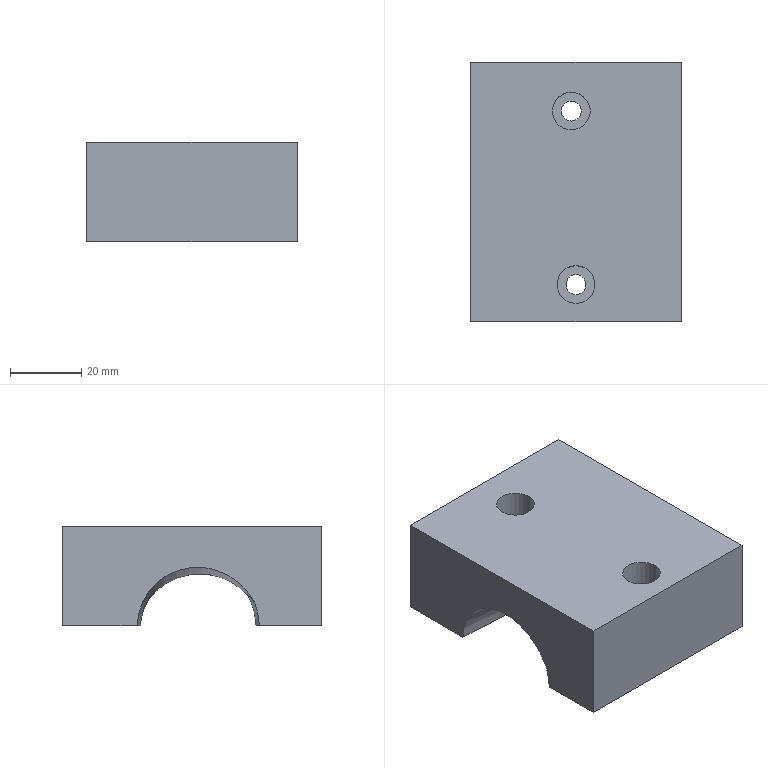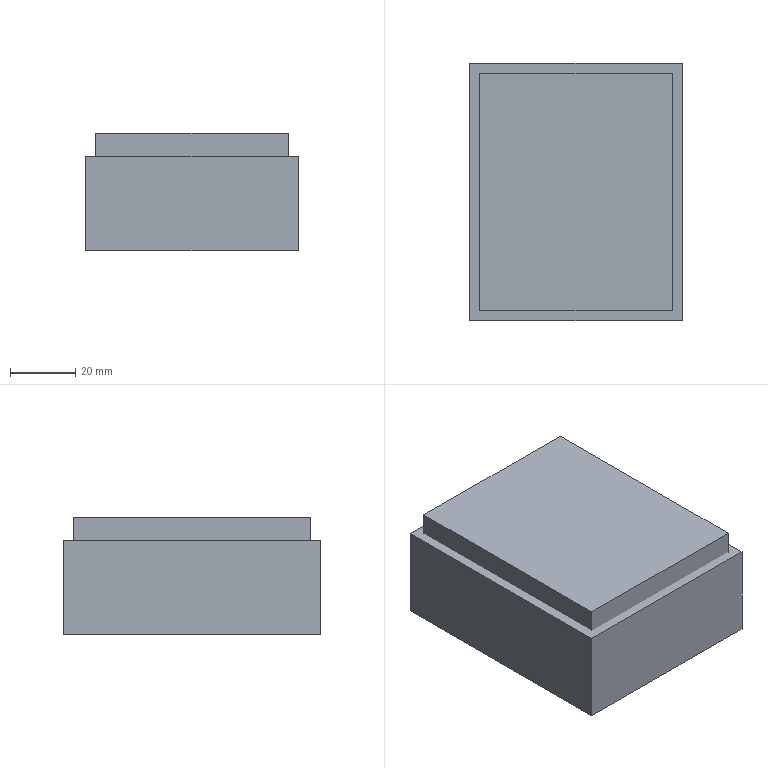CAM job | NX | 3-axis milling, drilling | part box 59.014 x 72.744 x 27.972 mm | stock box 65.014 x 78.744 x 35.972 mm
Tools:
number,name,description,diameter,corner_radius,flute_length,length,flutes
3,D63,Milling Tool-5 Parameters,63.0,0.0,50.0,75.0,2
1,D6A45,Milling Tool-5 Parameters,6.0,0.0,3.0,3.0,2
20,5.6ZT,Drilling Tool,5.6,0.0,35.0,50.0,2
16,D6,Milling Tool-5 Parameters,6.0,0.0,50.0,75.0,2
4,D10,Milling Tool-5 Parameters,10.0,0.0,50.0,75.0,2
14,D10JING,Milling Tool-5 Parameters,10.0,0.0,50.0,75.0,2
11,R2,Milling Tool-5 Parameters,4.0,2.0,50.0,75.0,2
Operations:
program,operation,operation_type,tool,method,geometry_group,spindle_rpm,surface_speed,feed_per_tooth,feed_cut,feed_plunge,cut_length_mm,path_length_mm,cut_time_min,machine_time_min
1,FLOOR_WALL,VolumeBased25DMillingOperation,D63,METHOD,A,6500.0,1286.0,0.1154,1500.0,100.0,153.744,207.744,0.1025,0.1079
1,DRILLING,Operation,D6A45,METHOD,A,5000.0,94.0,0.025,250.0,0.0,8.0,127.791,0.032,0.044
1,DRILLING_COPY_COPY,Operation,5.6ZT,METHOD,A,2000.0,37.0,0.0375,150.0,0.0,68.308,248.408,0.4554,0.4734
1,HOLE_MILLING,CylinderMilling,D6,METHOD,A,9500.0,179.0,0.0763,1450.0,100.0,1229.072,1436.771,0.8476,0.8684
1,ADAPTIVE_MILLING,CavityMilling,D10,METHOD,A,9500.0,298.0,0.1579,3000.0,1000.0,1303.741,1532.07,0.4386,0.4614
1,ZLEVEL_PROFILE_COPY_COPY,ZLevelMilling,D10JING,METHOD,A,9500.0,298.0,0.0632,1200.0,1000.0,596.127,712.251,0.4973,0.5089
1,ZLEVEL_PROFILE_1,ZLevelMilling,D6A45,METHOD,A,9500.0,179.0,0.0658,1250.0,100.0,344.132,617.739,0.2753,0.3027
2,FLOOR_WALL_COPY_1,VolumeBased25DMillingOperation,D63,METHOD,B,6500.0,1286.0,0.1154,1500.0,100.0,1181.948,2548.356,0.788,0.9246
2,FLOOR_WALL_COPY,VolumeBased25DMillingOperation,D63,METHOD,B,6500.0,1286.0,0.1154,1500.0,100.0,147.744,201.744,0.0985,0.1039
2,ZLEVEL_PROFILE,ZLevelMilling,D10,METHOD,B,9500.0,298.0,0.1579,3000.0,1000.0,5420.607,5895.56,1.827,1.875
2,ZLEVEL_PROFILE_COPY,ZLevelMilling,D6,METHOD,B,9500.0,179.0,0.1316,2500.0,1000.0,928.56,1871.983,0.4004,0.4947
2,FIXED_CONTOUR,SurfaceContour,R2,METHOD,B,9500.0,298.0,0.1579,3000.0,1000.0,50308.98,50358.58,16.773,16.778
2,ZLEVEL_PROFILE_1_COPY,ZLevelMilling,D6A45,METHOD,B,9500.0,179.0,0.0658,1250.0,100.0,411.126,952.935,0.3289,0.3831